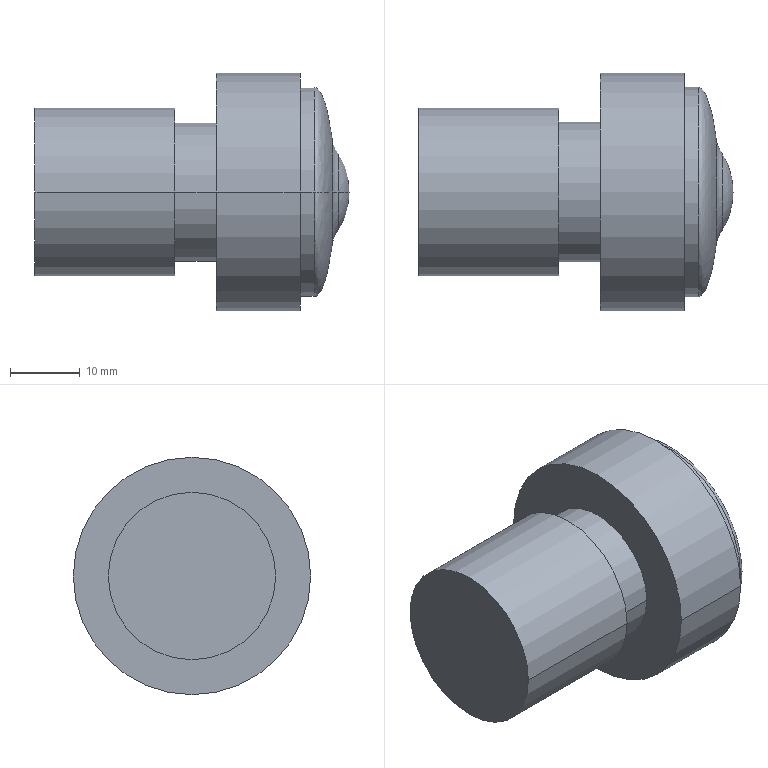Part | SolidWorks | features Revolution 1 | 1 solid | 18 faces | box 45 x 34 x 34 mm | volume 24801 mm3 | cylinder 8 | spline 4 | plane 4 | torus 2 | commonest cylinder face diameters 20 x2 24 x2 30 x2 34 x2
STEP:
#1=CARTESIAN_POINT('',(42.569,7.738,0.));
#2=VERTEX_POINT('',#1);
#3=CARTESIAN_POINT('',(42.569,-7.738,0.));
#4=VERTEX_POINT('',#3);
#5=CARTESIAN_POINT('',(42.569,0.,0.));
#6=DIRECTION('',(-1.,0.,0.));
#7=DIRECTION('',(0.,-1.,0.));
#8=AXIS2_PLACEMENT_3D('',#5,#6,#7);
#9=CIRCLE('',#8,7.738);
#10=EDGE_CURVE('',#2,#4,#9,.T.);
#11=ORIENTED_EDGE('',*,*,#10,.T.);
#12=CARTESIAN_POINT('',(39.999,-15.,0.));
#13=VERTEX_POINT('',#12);
#14=CARTESIAN_POINT('',(42.569,-7.738,0.));
#15=CARTESIAN_POINT('',(42.013,-12.351,0.));
#16=CARTESIAN_POINT('',(41.075,-15.,0.));
#17=CARTESIAN_POINT('',(39.999,-15.,0.));
#18=(BOUNDED_CURVE()B_SPLINE_CURVE(3,(#14,#15,#16,#17),.UNSPECIFIED.,.F.,.T.)B_SPLINE_CURVE_WITH_KNOTS((4,4),(5.254,6.283),.UNSPECIFIED.)CURVE()GEOMETRIC_REPRESENTATION_ITEM()RATIONAL_B_SPLINE_CURVE((1.,0.9137,0.9137,1.))REPRESENTATION_ITEM(''));
#19=EDGE_CURVE('',#4,#13,#18,.T.);
#20=ORIENTED_EDGE('',*,*,#19,.T.);
#21=CARTESIAN_POINT('',(39.999,15.,0.));
#22=VERTEX_POINT('',#21);
#23=CARTESIAN_POINT('',(39.999,0.,0.));
#24=DIRECTION('',(-1.,0.,0.));
#25=DIRECTION('',(0.,-1.,0.));
#26=AXIS2_PLACEMENT_3D('',#23,#24,#25);
#27=CIRCLE('',#26,15.);
#28=EDGE_CURVE('',#22,#13,#27,.T.);
#29=ORIENTED_EDGE('',*,*,#28,.F.);
#30=CARTESIAN_POINT('',(42.569,7.738,0.));
#31=CARTESIAN_POINT('',(42.013,12.351,0.));
#32=CARTESIAN_POINT('',(41.075,15.,0.));
#33=CARTESIAN_POINT('',(39.999,15.,0.));
#34=(BOUNDED_CURVE()B_SPLINE_CURVE(3,(#30,#31,#32,#33),.UNSPECIFIED.,.F.,.F.)B_SPLINE_CURVE_WITH_KNOTS((4,4),(5.254,6.283),.UNSPECIFIED.)CURVE()GEOMETRIC_REPRESENTATION_ITEM()RATIONAL_B_SPLINE_CURVE((1.,0.9137,0.9137,1.))REPRESENTATION_ITEM(''));
#35=EDGE_CURVE('',#2,#22,#34,.T.);
#36=ORIENTED_EDGE('',*,*,#35,.F.);
#37=EDGE_LOOP('',(#11,#20,#29,#36));
#38=FACE_OUTER_BOUND('',#37,.T.);
#39=CARTESIAN_POINT('',(42.569,7.738,0.));
#40=CARTESIAN_POINT('',(42.569,7.738,-15.476));
#41=CARTESIAN_POINT('',(42.569,-7.738,-15.476));
#42=CARTESIAN_POINT('',(42.569,-7.738,0.));
#43=CARTESIAN_POINT('',(42.013,12.351,0.));
#44=CARTESIAN_POINT('',(42.013,12.351,-24.702));
#45=CARTESIAN_POINT('',(42.013,-12.351,-24.702));
#46=CARTESIAN_POINT('',(42.013,-12.351,0.));
#47=CARTESIAN_POINT('',(41.075,15.,0.));
#48=CARTESIAN_POINT('',(41.075,15.,-30.));
#49=CARTESIAN_POINT('',(41.075,-15.,-30.));
#50=CARTESIAN_POINT('',(41.075,-15.,0.));
#51=CARTESIAN_POINT('',(39.999,15.,0.));
#52=CARTESIAN_POINT('',(39.999,15.,-30.));
#53=CARTESIAN_POINT('',(39.999,-15.,-30.));
#54=CARTESIAN_POINT('',(39.999,-15.,0.));
#55=(BOUNDED_SURFACE()B_SPLINE_SURFACE(3,3,((#39,#40,#41,#42),(#43,#44,#45,#46),(#47,#48,#49,#50),(#51,#52,#53,#54)),.UNSPECIFIED.,.F.,.F.,.T.)B_SPLINE_SURFACE_WITH_KNOTS((4,4),(4,4),(0.,1.),(0.,1.),.UNSPECIFIED.)GEOMETRIC_REPRESENTATION_ITEM()RATIONAL_B_SPLINE_SURFACE(((1.,0.3333,0.3333,1.),(0.9137,0.3046,0.3046,0.9137),(0.9137,0.3046,0.3046,0.9137),(1.,0.3333,0.3333,1.)))REPRESENTATION_ITEM('')SURFACE());
#56=ADVANCED_FACE('',(#38),#55,.F.);
#57=CARTESIAN_POINT('',(45.,0.,0.));
#58=VERTEX_POINT('',#57);
#59=CARTESIAN_POINT('',(43.439,5.466,0.));
#60=VERTEX_POINT('',#59);
#61=CARTESIAN_POINT('',(45.,0.,0.));
#62=CARTESIAN_POINT('',(45.,2.097,0.));
#63=CARTESIAN_POINT('',(44.45,4.023,0.));
#64=CARTESIAN_POINT('',(43.439,5.466,0.));
#65=(BOUNDED_CURVE()B_SPLINE_CURVE(3,(#61,#62,#63,#64),.UNSPECIFIED.,.F.,.F.)B_SPLINE_CURVE_WITH_KNOTS((4,4),(4.712,5.525),.UNSPECIFIED.)CURVE()GEOMETRIC_REPRESENTATION_ITEM()RATIONAL_B_SPLINE_CURVE((1.,0.9458,0.9458,1.))REPRESENTATION_ITEM(''));
#66=EDGE_CURVE('',#58,#60,#65,.T.);
#67=ORIENTED_EDGE('',*,*,#66,.F.);
#68=CARTESIAN_POINT('',(43.439,-5.466,0.));
#69=VERTEX_POINT('',#68);
#70=CARTESIAN_POINT('',(45.,0.,0.));
#71=CARTESIAN_POINT('',(45.,-2.097,0.));
#72=CARTESIAN_POINT('',(44.45,-4.023,0.));
#73=CARTESIAN_POINT('',(43.439,-5.466,0.));
#74=(BOUNDED_CURVE()B_SPLINE_CURVE(3,(#70,#71,#72,#73),.UNSPECIFIED.,.F.,.F.)B_SPLINE_CURVE_WITH_KNOTS((4,4),(4.712,5.525),.UNSPECIFIED.)CURVE()GEOMETRIC_REPRESENTATION_ITEM()RATIONAL_B_SPLINE_CURVE((1.,0.9458,0.9458,1.))REPRESENTATION_ITEM(''));
#75=EDGE_CURVE('',#58,#69,#74,.T.);
#76=ORIENTED_EDGE('',*,*,#75,.T.);
#77=CARTESIAN_POINT('',(43.439,0.,0.));
#78=DIRECTION('',(-1.,0.,0.));
#79=DIRECTION('',(0.,-1.,0.));
#80=AXIS2_PLACEMENT_3D('',#77,#78,#79);
#81=CIRCLE('',#80,5.466);
#82=EDGE_CURVE('',#60,#69,#81,.T.);
#83=ORIENTED_EDGE('',*,*,#82,.F.);
#84=EDGE_LOOP('',(#67,#76,#83));
#85=FACE_OUTER_BOUND('',#84,.T.);
#86=CARTESIAN_POINT('',(45.,0.,0.));
#87=CARTESIAN_POINT('',(45.,0.,0.));
#88=CARTESIAN_POINT('',(45.,0.,0.));
#89=CARTESIAN_POINT('',(45.,0.,0.));
#90=CARTESIAN_POINT('',(45.,2.097,0.));
#91=CARTESIAN_POINT('',(45.,2.097,-4.194));
#92=CARTESIAN_POINT('',(45.,-2.097,-4.194));
#93=CARTESIAN_POINT('',(45.,-2.097,0.));
#94=CARTESIAN_POINT('',(44.45,4.023,0.));
#95=CARTESIAN_POINT('',(44.45,4.023,-8.047));
#96=CARTESIAN_POINT('',(44.45,-4.023,-8.047));
#97=CARTESIAN_POINT('',(44.45,-4.023,0.));
#98=CARTESIAN_POINT('',(43.439,5.466,0.));
#99=CARTESIAN_POINT('',(43.439,5.466,-10.931));
#100=CARTESIAN_POINT('',(43.439,-5.466,-10.931));
#101=CARTESIAN_POINT('',(43.439,-5.466,0.));
#102=(BOUNDED_SURFACE()B_SPLINE_SURFACE(3,3,((#86,#87,#88,#89),(#90,#91,#92,#93),(#94,#95,#96,#97),(#98,#99,#100,#101)),.UNSPECIFIED.,.F.,.F.,.T.)B_SPLINE_SURFACE_WITH_KNOTS((4,4),(4,4),(0.,1.),(0.,1.),.UNSPECIFIED.)GEOMETRIC_REPRESENTATION_ITEM()RATIONAL_B_SPLINE_SURFACE(((1.,0.3333,0.3333,1.),(0.9458,0.3153,0.3153,0.9458),(0.9458,0.3153,0.3153,0.9458),(1.,0.3333,0.3333,1.)))REPRESENTATION_ITEM('')SURFACE());
#103=ADVANCED_FACE('',(#85),#102,.F.);
#104=CARTESIAN_POINT('',(20.,-12.,0.));
#105=VERTEX_POINT('',#104);
#106=CARTESIAN_POINT('',(20.,12.,0.));
#107=VERTEX_POINT('',#106);
#108=CARTESIAN_POINT('',(20.,0.,0.));
#109=DIRECTION('',(-1.,0.,0.));
#110=DIRECTION('',(0.,-1.,0.));
#111=AXIS2_PLACEMENT_3D('',#108,#109,#110);
#112=CIRCLE('',#111,12.);
#113=EDGE_CURVE('',#105,#107,#112,.T.);
#114=ORIENTED_EDGE('',*,*,#113,.T.);
#115=CARTESIAN_POINT('',(0.,12.,0.));
#116=VERTEX_POINT('',#115);
#117=CARTESIAN_POINT('',(0.,12.,0.));
#118=DIRECTION('',(-1.,0.,0.));
#119=VECTOR('',#118,1000.);
#120=LINE('',#117,#119);
#121=EDGE_CURVE('',#107,#116,#120,.T.);
#122=ORIENTED_EDGE('',*,*,#121,.T.);
#123=CARTESIAN_POINT('',(0.,-12.,0.));
#124=VERTEX_POINT('',#123);
#125=CARTESIAN_POINT('',(0.,0.,0.));
#126=DIRECTION('',(-1.,0.,0.));
#127=DIRECTION('',(0.,-1.,0.));
#128=AXIS2_PLACEMENT_3D('',#125,#126,#127);
#129=CIRCLE('',#128,12.);
#130=EDGE_CURVE('',#124,#116,#129,.T.);
#131=ORIENTED_EDGE('',*,*,#130,.F.);
#132=CARTESIAN_POINT('',(0.,-12.,0.));
#133=DIRECTION('',(-1.,0.,0.));
#134=VECTOR('',#133,1000.);
#135=LINE('',#132,#134);
#136=EDGE_CURVE('',#105,#124,#135,.T.);
#137=ORIENTED_EDGE('',*,*,#136,.F.);
#138=EDGE_LOOP('',(#114,#122,#131,#137));
#139=FACE_OUTER_BOUND('',#138,.T.);
#140=CARTESIAN_POINT('',(0.,0.,0.));
#141=DIRECTION('',(-1.,0.,0.));
#142=DIRECTION('',(0.,-1.,0.));
#143=AXIS2_PLACEMENT_3D('',#140,#141,#142);
#144=CYLINDRICAL_SURFACE('',#143,12.);
#145=ADVANCED_FACE('',(#139),#144,.T.);
#146=CARTESIAN_POINT('',(25.999,-10.,0.));
#147=VERTEX_POINT('',#146);
#148=CARTESIAN_POINT('',(25.999,10.,0.));
#149=VERTEX_POINT('',#148);
#150=CARTESIAN_POINT('',(25.999,0.,0.));
#151=DIRECTION('',(-1.,0.,0.));
#152=DIRECTION('',(0.,-1.,0.));
#153=AXIS2_PLACEMENT_3D('',#150,#151,#152);
#154=CIRCLE('',#153,10.);
#155=EDGE_CURVE('',#147,#149,#154,.T.);
#156=ORIENTED_EDGE('',*,*,#155,.T.);
#157=CARTESIAN_POINT('',(20.,10.,0.));
#158=VERTEX_POINT('',#157);
#159=CARTESIAN_POINT('',(0.,10.,0.));
#160=DIRECTION('',(-1.,0.,0.));
#161=VECTOR('',#160,1000.);
#162=LINE('',#159,#161);
#163=EDGE_CURVE('',#149,#158,#162,.T.);
#164=ORIENTED_EDGE('',*,*,#163,.T.);
#165=CARTESIAN_POINT('',(20.,-10.,0.));
#166=VERTEX_POINT('',#165);
#167=CARTESIAN_POINT('',(20.,0.,0.));
#168=DIRECTION('',(-1.,0.,0.));
#169=DIRECTION('',(0.,-1.,0.));
#170=AXIS2_PLACEMENT_3D('',#167,#168,#169);
#171=CIRCLE('',#170,10.);
#172=EDGE_CURVE('',#166,#158,#171,.T.);
#173=ORIENTED_EDGE('',*,*,#172,.F.);
#174=CARTESIAN_POINT('',(0.,-10.,0.));
#175=DIRECTION('',(-1.,0.,0.));
#176=VECTOR('',#175,1000.);
#177=LINE('',#174,#176);
#178=EDGE_CURVE('',#147,#166,#177,.T.);
#179=ORIENTED_EDGE('',*,*,#178,.F.);
#180=EDGE_LOOP('',(#156,#164,#173,#179));
#181=FACE_OUTER_BOUND('',#180,.T.);
#182=CARTESIAN_POINT('',(0.,0.,0.));
#183=DIRECTION('',(-1.,0.,0.));
#184=DIRECTION('',(0.,-1.,0.));
#185=AXIS2_PLACEMENT_3D('',#182,#183,#184);
#186=CYLINDRICAL_SURFACE('',#185,10.);
#187=ADVANCED_FACE('',(#181),#186,.T.);
#188=CARTESIAN_POINT('',(37.999,-17.,0.));
#189=VERTEX_POINT('',#188);
#190=CARTESIAN_POINT('',(37.999,17.,0.));
#191=VERTEX_POINT('',#190);
#192=CARTESIAN_POINT('',(37.999,0.,0.));
#193=DIRECTION('',(-1.,0.,0.));
#194=DIRECTION('',(0.,-1.,0.));
#195=AXIS2_PLACEMENT_3D('',#192,#193,#194);
#196=CIRCLE('',#195,17.);
#197=EDGE_CURVE('',#189,#191,#196,.T.);
#198=ORIENTED_EDGE('',*,*,#197,.T.);
#199=CARTESIAN_POINT('',(25.999,17.,0.));
#200=VERTEX_POINT('',#199);
#201=CARTESIAN_POINT('',(0.,17.,0.));
#202=DIRECTION('',(-1.,0.,0.));
#203=VECTOR('',#202,1000.);
#204=LINE('',#201,#203);
#205=EDGE_CURVE('',#191,#200,#204,.T.);
#206=ORIENTED_EDGE('',*,*,#205,.T.);
#207=CARTESIAN_POINT('',(25.999,-17.,0.));
#208=VERTEX_POINT('',#207);
#209=CARTESIAN_POINT('',(25.999,0.,0.));
#210=DIRECTION('',(-1.,0.,0.));
#211=DIRECTION('',(0.,-1.,0.));
#212=AXIS2_PLACEMENT_3D('',#209,#210,#211);
#213=CIRCLE('',#212,17.);
#214=EDGE_CURVE('',#208,#200,#213,.T.);
#215=ORIENTED_EDGE('',*,*,#214,.F.);
#216=CARTESIAN_POINT('',(0.,-17.,0.));
#217=DIRECTION('',(-1.,0.,0.));
#218=VECTOR('',#217,1000.);
#219=LINE('',#216,#218);
#220=EDGE_CURVE('',#189,#208,#219,.T.);
#221=ORIENTED_EDGE('',*,*,#220,.F.);
#222=EDGE_LOOP('',(#198,#206,#215,#221));
#223=FACE_OUTER_BOUND('',#222,.T.);
#224=CARTESIAN_POINT('',(0.,0.,0.));
#225=DIRECTION('',(-1.,0.,0.));
#226=DIRECTION('',(0.,-1.,0.));
#227=AXIS2_PLACEMENT_3D('',#224,#225,#226);
#228=CYLINDRICAL_SURFACE('',#227,17.);
#229=ADVANCED_FACE('',(#223),#228,.T.);
#230=CARTESIAN_POINT('',(39.999,0.,0.));
#231=DIRECTION('',(-1.,0.,0.));
#232=DIRECTION('',(0.,-1.,0.));
#233=AXIS2_PLACEMENT_3D('',#230,#231,#232);
#234=CIRCLE('',#233,15.);
#235=EDGE_CURVE('',#13,#22,#234,.T.);
#236=ORIENTED_EDGE('',*,*,#235,.T.);
#237=CARTESIAN_POINT('',(37.999,15.,0.));
#238=VERTEX_POINT('',#237);
#239=CARTESIAN_POINT('',(0.,15.,0.));
#240=DIRECTION('',(-1.,0.,0.));
#241=VECTOR('',#240,1000.);
#242=LINE('',#239,#241);
#243=EDGE_CURVE('',#22,#238,#242,.T.);
#244=ORIENTED_EDGE('',*,*,#243,.T.);
#245=CARTESIAN_POINT('',(37.999,-15.,0.));
#246=VERTEX_POINT('',#245);
#247=CARTESIAN_POINT('',(37.999,0.,0.));
#248=DIRECTION('',(-1.,0.,0.));
#249=DIRECTION('',(0.,-1.,0.));
#250=AXIS2_PLACEMENT_3D('',#247,#248,#249);
#251=CIRCLE('',#250,15.);
#252=EDGE_CURVE('',#246,#238,#251,.T.);
#253=ORIENTED_EDGE('',*,*,#252,.F.);
#254=CARTESIAN_POINT('',(0.,-15.,0.));
#255=DIRECTION('',(-1.,0.,0.));
#256=VECTOR('',#255,1000.);
#257=LINE('',#254,#256);
#258=EDGE_CURVE('',#13,#246,#257,.T.);
#259=ORIENTED_EDGE('',*,*,#258,.F.);
#260=EDGE_LOOP('',(#236,#244,#253,#259));
#261=FACE_OUTER_BOUND('',#260,.T.);
#262=CARTESIAN_POINT('',(0.,0.,0.));
#263=DIRECTION('',(-1.,0.,0.));
#264=DIRECTION('',(0.,-1.,0.));
#265=AXIS2_PLACEMENT_3D('',#262,#263,#264);
#266=CYLINDRICAL_SURFACE('',#265,15.);
#267=ADVANCED_FACE('',(#261),#266,.T.);
#268=ORIENTED_EDGE('',*,*,#10,.F.);
#269=CARTESIAN_POINT('',(47.533,8.336,0.));
#270=DIRECTION('',(0.,0.,1.));
#271=DIRECTION('',(0.,-1.,0.));
#272=AXIS2_PLACEMENT_3D('',#269,#270,#271);
#273=CIRCLE('',#272,5.);
#274=EDGE_CURVE('',#2,#60,#273,.T.);
#275=ORIENTED_EDGE('',*,*,#274,.T.);
#276=ORIENTED_EDGE('',*,*,#82,.T.);
#277=CARTESIAN_POINT('',(47.533,-8.336,0.));
#278=DIRECTION('',(0.,0.,-1.));
#279=DIRECTION('',(-1.,0.,0.));
#280=AXIS2_PLACEMENT_3D('',#277,#278,#279);
#281=CIRCLE('',#280,5.);
#282=EDGE_CURVE('',#4,#69,#281,.T.);
#283=ORIENTED_EDGE('',*,*,#282,.F.);
#284=EDGE_LOOP('',(#268,#275,#276,#283));
#285=FACE_OUTER_BOUND('',#284,.T.);
#286=CARTESIAN_POINT('',(47.533,0.,0.));
#287=DIRECTION('',(-1.,0.,0.));
#288=DIRECTION('',(0.,-1.,0.));
#289=AXIS2_PLACEMENT_3D('',#286,#287,#288);
#290=TOROIDAL_SURFACE('',#289,8.336,5.);
#291=ADVANCED_FACE('',(#285),#290,.F.);
#292=ORIENTED_EDGE('',*,*,#75,.F.);
#293=ORIENTED_EDGE('',*,*,#66,.T.);
#294=CARTESIAN_POINT('',(43.439,0.,0.));
#295=DIRECTION('',(-1.,0.,0.));
#296=DIRECTION('',(0.,-1.,0.));
#297=AXIS2_PLACEMENT_3D('',#294,#295,#296);
#298=CIRCLE('',#297,5.466);
#299=EDGE_CURVE('',#69,#60,#298,.T.);
#300=ORIENTED_EDGE('',*,*,#299,.F.);
#301=EDGE_LOOP('',(#292,#293,#300));
#302=FACE_OUTER_BOUND('',#301,.T.);
#303=CARTESIAN_POINT('',(45.,0.,0.));
#304=CARTESIAN_POINT('',(45.,0.,0.));
#305=CARTESIAN_POINT('',(45.,0.,0.));
#306=CARTESIAN_POINT('',(45.,0.,0.));
#307=CARTESIAN_POINT('',(45.,-2.097,0.));
#308=CARTESIAN_POINT('',(45.,-2.097,4.194));
#309=CARTESIAN_POINT('',(45.,2.097,4.194));
#310=CARTESIAN_POINT('',(45.,2.097,0.));
#311=CARTESIAN_POINT('',(44.45,-4.023,0.));
#312=CARTESIAN_POINT('',(44.45,-4.023,8.047));
#313=CARTESIAN_POINT('',(44.45,4.023,8.047));
#314=CARTESIAN_POINT('',(44.45,4.023,0.));
#315=CARTESIAN_POINT('',(43.439,-5.466,0.));
#316=CARTESIAN_POINT('',(43.439,-5.466,10.931));
#317=CARTESIAN_POINT('',(43.439,5.466,10.931));
#318=CARTESIAN_POINT('',(43.439,5.466,0.));
#319=(BOUNDED_SURFACE()B_SPLINE_SURFACE(3,3,((#303,#304,#305,#306),(#307,#308,#309,#310),(#311,#312,#313,#314),(#315,#316,#317,#318)),.UNSPECIFIED.,.F.,.F.,.F.)B_SPLINE_SURFACE_WITH_KNOTS((4,4),(4,4),(0.,1.),(0.,1.),.UNSPECIFIED.)GEOMETRIC_REPRESENTATION_ITEM()RATIONAL_B_SPLINE_SURFACE(((1.,0.3333,0.3333,1.),(0.9458,0.3153,0.3153,0.9458),(0.9458,0.3153,0.3153,0.9458),(1.,0.3333,0.3333,1.)))REPRESENTATION_ITEM('')SURFACE());
#320=ADVANCED_FACE('',(#302),#319,.F.);
#321=ORIENTED_EDGE('',*,*,#274,.F.);
#322=CARTESIAN_POINT('',(42.569,0.,0.));
#323=DIRECTION('',(-1.,0.,0.));
#324=DIRECTION('',(0.,-1.,0.));
#325=AXIS2_PLACEMENT_3D('',#322,#323,#324);
#326=CIRCLE('',#325,7.738);
#327=EDGE_CURVE('',#4,#2,#326,.T.);
#328=ORIENTED_EDGE('',*,*,#327,.F.);
#329=ORIENTED_EDGE('',*,*,#282,.T.);
#330=ORIENTED_EDGE('',*,*,#299,.T.);
#331=EDGE_LOOP('',(#321,#328,#329,#330));
#332=FACE_OUTER_BOUND('',#331,.T.);
#333=CARTESIAN_POINT('',(47.533,0.,0.));
#334=DIRECTION('',(-1.,0.,0.));
#335=DIRECTION('',(0.,-1.,0.));
#336=AXIS2_PLACEMENT_3D('',#333,#334,#335);
#337=TOROIDAL_SURFACE('',#336,8.336,5.);
#338=ADVANCED_FACE('',(#332),#337,.F.);
#339=ORIENTED_EDGE('',*,*,#19,.F.);
#340=ORIENTED_EDGE('',*,*,#327,.T.);
#341=ORIENTED_EDGE('',*,*,#35,.T.);
#342=ORIENTED_EDGE('',*,*,#235,.F.);
#343=EDGE_LOOP('',(#339,#340,#341,#342));
#344=FACE_OUTER_BOUND('',#343,.T.);
#345=CARTESIAN_POINT('',(42.569,-7.738,0.));
#346=CARTESIAN_POINT('',(42.569,-7.738,15.476));
#347=CARTESIAN_POINT('',(42.569,7.738,15.476));
#348=CARTESIAN_POINT('',(42.569,7.738,0.));
#349=CARTESIAN_POINT('',(42.013,-12.351,0.));
#350=CARTESIAN_POINT('',(42.013,-12.351,24.702));
#351=CARTESIAN_POINT('',(42.013,12.351,24.702));
#352=CARTESIAN_POINT('',(42.013,12.351,0.));
#353=CARTESIAN_POINT('',(41.075,-15.,0.));
#354=CARTESIAN_POINT('',(41.075,-15.,30.));
#355=CARTESIAN_POINT('',(41.075,15.,30.));
#356=CARTESIAN_POINT('',(41.075,15.,0.));
#357=CARTESIAN_POINT('',(39.999,-15.,0.));
#358=CARTESIAN_POINT('',(39.999,-15.,30.));
#359=CARTESIAN_POINT('',(39.999,15.,30.));
#360=CARTESIAN_POINT('',(39.999,15.,0.));
#361=(BOUNDED_SURFACE()B_SPLINE_SURFACE(3,3,((#345,#346,#347,#348),(#349,#350,#351,#352),(#353,#354,#355,#356),(#357,#358,#359,#360)),.UNSPECIFIED.,.F.,.F.,.F.)B_SPLINE_SURFACE_WITH_KNOTS((4,4),(4,4),(0.,1.),(0.,1.),.UNSPECIFIED.)GEOMETRIC_REPRESENTATION_ITEM()RATIONAL_B_SPLINE_SURFACE(((1.,0.3333,0.3333,1.),(0.9137,0.3046,0.3046,0.9137),(0.9137,0.3046,0.3046,0.9137),(1.,0.3333,0.3333,1.)))REPRESENTATION_ITEM('')SURFACE());
#362=ADVANCED_FACE('',(#344),#361,.F.);
#363=ORIENTED_EDGE('',*,*,#243,.F.);
#364=ORIENTED_EDGE('',*,*,#28,.T.);
#365=ORIENTED_EDGE('',*,*,#258,.T.);
#366=CARTESIAN_POINT('',(37.999,0.,0.));
#367=DIRECTION('',(-1.,0.,0.));
#368=DIRECTION('',(0.,-1.,0.));
#369=AXIS2_PLACEMENT_3D('',#366,#367,#368);
#370=CIRCLE('',#369,15.);
#371=EDGE_CURVE('',#238,#246,#370,.T.);
#372=ORIENTED_EDGE('',*,*,#371,.F.);
#373=EDGE_LOOP('',(#363,#364,#365,#372));
#374=FACE_OUTER_BOUND('',#373,.T.);
#375=CARTESIAN_POINT('',(0.,0.,0.));
#376=DIRECTION('',(-1.,0.,0.));
#377=DIRECTION('',(0.,-1.,0.));
#378=AXIS2_PLACEMENT_3D('',#375,#376,#377);
#379=CYLINDRICAL_SURFACE('',#378,15.);
#380=ADVANCED_FACE('',(#374),#379,.T.);
#381=ORIENTED_EDGE('',*,*,#197,.F.);
#382=CARTESIAN_POINT('',(37.999,0.,0.));
#383=DIRECTION('',(-1.,0.,0.));
#384=DIRECTION('',(0.,-1.,0.));
#385=AXIS2_PLACEMENT_3D('',#382,#383,#384);
#386=CIRCLE('',#385,17.);
#387=EDGE_CURVE('',#191,#189,#386,.T.);
#388=ORIENTED_EDGE('',*,*,#387,.F.);
#389=EDGE_LOOP('',(#381,#388));
#390=FACE_OUTER_BOUND('',#389,.T.);
#391=ORIENTED_EDGE('',*,*,#252,.T.);
#392=ORIENTED_EDGE('',*,*,#371,.T.);
#393=EDGE_LOOP('',(#391,#392));
#394=FACE_BOUND('',#393,.T.);
#395=CARTESIAN_POINT('',(37.999,17.,0.));
#396=DIRECTION('',(-1.,0.,0.));
#397=DIRECTION('',(0.,-1.,0.));
#398=AXIS2_PLACEMENT_3D('',#395,#396,#397);
#399=PLANE('',#398);
#400=ADVANCED_FACE('',(#390,#394),#399,.F.);
#401=ORIENTED_EDGE('',*,*,#205,.F.);
#402=ORIENTED_EDGE('',*,*,#387,.T.);
#403=ORIENTED_EDGE('',*,*,#220,.T.);
#404=CARTESIAN_POINT('',(25.999,0.,0.));
#405=DIRECTION('',(-1.,0.,0.));
#406=DIRECTION('',(0.,-1.,0.));
#407=AXIS2_PLACEMENT_3D('',#404,#405,#406);
#408=CIRCLE('',#407,17.);
#409=EDGE_CURVE('',#200,#208,#408,.T.);
#410=ORIENTED_EDGE('',*,*,#409,.F.);
#411=EDGE_LOOP('',(#401,#402,#403,#410));
#412=FACE_OUTER_BOUND('',#411,.T.);
#413=CARTESIAN_POINT('',(0.,0.,0.));
#414=DIRECTION('',(-1.,0.,0.));
#415=DIRECTION('',(0.,-1.,0.));
#416=AXIS2_PLACEMENT_3D('',#413,#414,#415);
#417=CYLINDRICAL_SURFACE('',#416,17.);
#418=ADVANCED_FACE('',(#412),#417,.T.);
#419=ORIENTED_EDGE('',*,*,#155,.F.);
#420=CARTESIAN_POINT('',(25.999,0.,0.));
#421=DIRECTION('',(-1.,0.,0.));
#422=DIRECTION('',(0.,-1.,0.));
#423=AXIS2_PLACEMENT_3D('',#420,#421,#422);
#424=CIRCLE('',#423,10.);
#425=EDGE_CURVE('',#149,#147,#424,.T.);
#426=ORIENTED_EDGE('',*,*,#425,.F.);
#427=EDGE_LOOP('',(#419,#426));
#428=FACE_BOUND('',#427,.T.);
#429=ORIENTED_EDGE('',*,*,#214,.T.);
#430=ORIENTED_EDGE('',*,*,#409,.T.);
#431=EDGE_LOOP('',(#429,#430));
#432=FACE_OUTER_BOUND('',#431,.T.);
#433=CARTESIAN_POINT('',(25.999,10.,0.));
#434=DIRECTION('',(1.,0.,0.));
#435=DIRECTION('',(0.,1.,0.));
#436=AXIS2_PLACEMENT_3D('',#433,#434,#435);
#437=PLANE('',#436);
#438=ADVANCED_FACE('',(#428,#432),#437,.F.);
#439=ORIENTED_EDGE('',*,*,#163,.F.);
#440=ORIENTED_EDGE('',*,*,#425,.T.);
#441=ORIENTED_EDGE('',*,*,#178,.T.);
#442=CARTESIAN_POINT('',(20.,0.,0.));
#443=DIRECTION('',(-1.,0.,0.));
#444=DIRECTION('',(0.,-1.,0.));
#445=AXIS2_PLACEMENT_3D('',#442,#443,#444);
#446=CIRCLE('',#445,10.);
#447=EDGE_CURVE('',#158,#166,#446,.T.);
#448=ORIENTED_EDGE('',*,*,#447,.F.);
#449=EDGE_LOOP('',(#439,#440,#441,#448));
#450=FACE_OUTER_BOUND('',#449,.T.);
#451=CARTESIAN_POINT('',(0.,0.,0.));
#452=DIRECTION('',(-1.,0.,0.));
#453=DIRECTION('',(0.,-1.,0.));
#454=AXIS2_PLACEMENT_3D('',#451,#452,#453);
#455=CYLINDRICAL_SURFACE('',#454,10.);
#456=ADVANCED_FACE('',(#450),#455,.T.);
#457=ORIENTED_EDGE('',*,*,#113,.F.);
#458=CARTESIAN_POINT('',(20.,0.,0.));
#459=DIRECTION('',(-1.,0.,0.));
#460=DIRECTION('',(0.,-1.,0.));
#461=AXIS2_PLACEMENT_3D('',#458,#459,#460);
#462=CIRCLE('',#461,12.);
#463=EDGE_CURVE('',#107,#105,#462,.T.);
#464=ORIENTED_EDGE('',*,*,#463,.F.);
#465=EDGE_LOOP('',(#457,#464));
#466=FACE_OUTER_BOUND('',#465,.T.);
#467=ORIENTED_EDGE('',*,*,#172,.T.);
#468=ORIENTED_EDGE('',*,*,#447,.T.);
#469=EDGE_LOOP('',(#467,#468));
#470=FACE_BOUND('',#469,.T.);
#471=CARTESIAN_POINT('',(20.,12.,0.));
#472=DIRECTION('',(-1.,0.,0.));
#473=DIRECTION('',(0.,-1.,0.));
#474=AXIS2_PLACEMENT_3D('',#471,#472,#473);
#475=PLANE('',#474);
#476=ADVANCED_FACE('',(#466,#470),#475,.F.);
#477=ORIENTED_EDGE('',*,*,#121,.F.);
#478=ORIENTED_EDGE('',*,*,#463,.T.);
#479=ORIENTED_EDGE('',*,*,#136,.T.);
#480=CARTESIAN_POINT('',(0.,0.,0.));
#481=DIRECTION('',(-1.,0.,0.));
#482=DIRECTION('',(0.,-1.,0.));
#483=AXIS2_PLACEMENT_3D('',#480,#481,#482);
#484=CIRCLE('',#483,12.);
#485=EDGE_CURVE('',#116,#124,#484,.T.);
#486=ORIENTED_EDGE('',*,*,#485,.F.);
#487=EDGE_LOOP('',(#477,#478,#479,#486));
#488=FACE_OUTER_BOUND('',#487,.T.);
#489=CARTESIAN_POINT('',(0.,0.,0.));
#490=DIRECTION('',(-1.,0.,0.));
#491=DIRECTION('',(0.,-1.,0.));
#492=AXIS2_PLACEMENT_3D('',#489,#490,#491);
#493=CYLINDRICAL_SURFACE('',#492,12.);
#494=ADVANCED_FACE('',(#488),#493,.T.);
#495=ORIENTED_EDGE('',*,*,#130,.T.);
#496=ORIENTED_EDGE('',*,*,#485,.T.);
#497=EDGE_LOOP('',(#495,#496));
#498=FACE_OUTER_BOUND('',#497,.T.);
#499=CARTESIAN_POINT('',(0.,0.,0.));
#500=DIRECTION('',(1.,0.,0.));
#501=DIRECTION('',(0.,1.,0.));
#502=AXIS2_PLACEMENT_3D('',#499,#500,#501);
#503=PLANE('',#502);
#504=ADVANCED_FACE('',(#498),#503,.F.);
#505=CLOSED_SHELL('',(#56,#103,#145,#187,#229,#267,#291,#320,#338,#362,#380,#400,#418,#438,#456,#476,#494,#504));
#506=MANIFOLD_SOLID_BREP('',#505);
#507=CARTESIAN_POINT('',(0.,0.,0.));
#508=DIRECTION('',(0.,0.,1.));
#509=DIRECTION('',(1.,0.,0.));
#510=AXIS2_PLACEMENT_3D('',#507,#508,#509);
#511=(LENGTH_UNIT()NAMED_UNIT(*)SI_UNIT(.MILLI.,.METRE.));
#512=UNCERTAINTY_MEASURE_WITH_UNIT(LENGTH_MEASURE(0.00001),#511,'','');
#513=(NAMED_UNIT(*)PLANE_ANGLE_UNIT()SI_UNIT($,.RADIAN.));
#514=(NAMED_UNIT(*)SI_UNIT($,.STERADIAN.)SOLID_ANGLE_UNIT());
#515=(GEOMETRIC_REPRESENTATION_CONTEXT(3)GLOBAL_UNCERTAINTY_ASSIGNED_CONTEXT((#512))GLOBAL_UNIT_ASSIGNED_CONTEXT((#511,#513,#514))REPRESENTATION_CONTEXT('',''));
#516=ADVANCED_BREP_SHAPE_REPRESENTATION('',(#506,#510),#515);